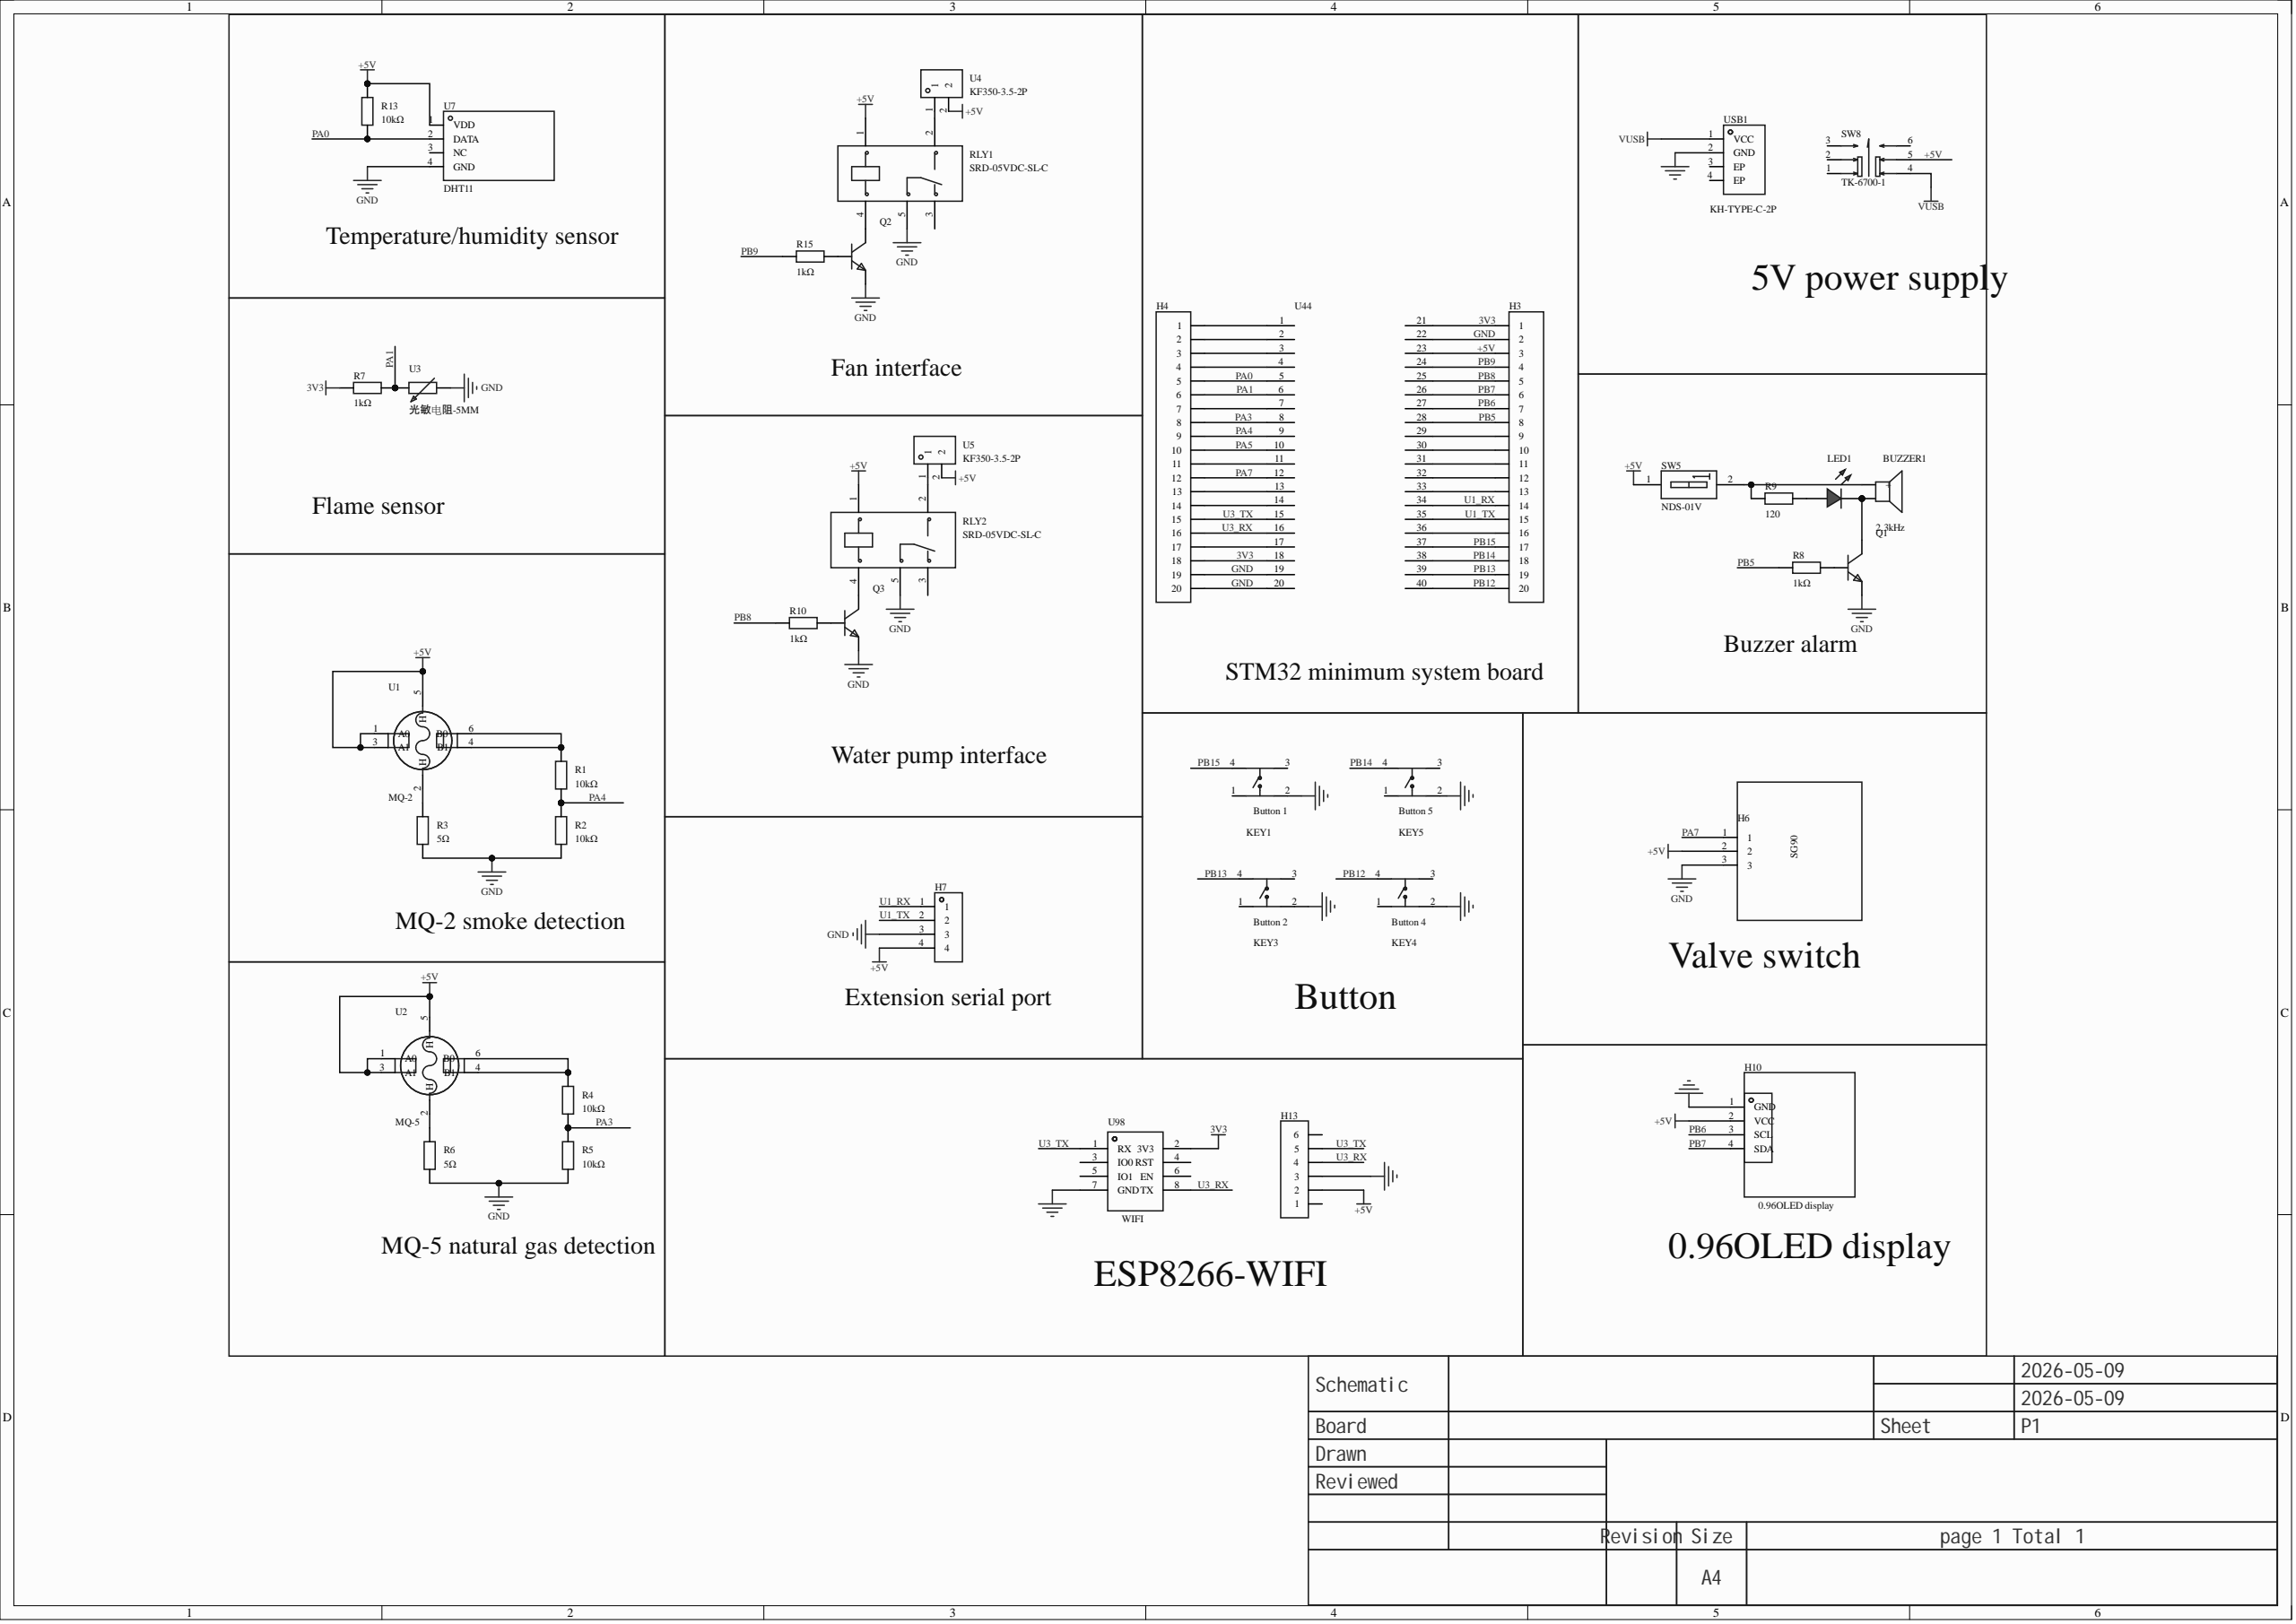Circuit board | Altium Designer | 40 parts | 52 nets
Bill of materials:
Comment,Description,Designator,Footprint,LibRef,Quantity
"2.3kHz","Drive mode: active (built-in driver circuit); construction type: electromagnetic; rated voltage: 5V; frequency: 2.3kHz; sound pressure (SPL): 85dB@5V,10cm;","BUZZER1","BUZ-TH_BD12.0-P7.60-D0.6-FD","TMB12A05_C96093","1"
"","","H3, H4","HDR-TH_20P-P2.54-V-F","HDR-F_2.54_1x20P","2"
"","","H6","HDR-TH_3P-P2.54-V-F","HDR-F_2.54_1x3P","1"
"","","H7","HDR-TH_4P-P2.54-V-F","HDR-F_2.54_1x4P","1"
"2.54-1*4P female","","H10","HDR-TH_4P-P2.54-V-F","0.96OLED屏幕","1"
"","","H13","HDR-TH_6P-P2.54-V-M-1","HDR-M_2.54_1x6P","1"
"Button 1","Circuit structure: SPST; contact rated current: -; button head type: Round Button; button actuation direction: Top Actuated;","KEY1","KEY-TH_4P-L6.0-W6.0-P4.50-LS7.5","按键开关6*6*8","1"
"Button 2","Circuit structure: SPST; contact rated current: -; button head type: Round Button; button actuation direction: Top Actuated;","KEY3","KEY-TH_4P-L6.0-W6.0-P4.50-LS7.5","按键开关6*6*8","1"
"Button 4","Circuit structure: SPST; contact rated current: -; button head type: Round Button; button actuation direction: Top Actuated;","KEY4","KEY-TH_4P-L6.0-W6.0-P4.50-LS7.5","按键开关6*6*8","1"
"Button 5","Circuit structure: SPST; contact rated current: -; button head type: Round Button; button actuation direction: Top Actuated;","KEY5","KEY-TH_4P-L6.0-W6.0-P4.50-LS7.5","按键开关6*6*8","1"
"","","LED1","LED_TH-3mm","LED_TH-R_3mm","1"
"","","Q1, Q2, Q3","S8050_TO_92","S8050_TO_NPN","3"
"10kΩ","","R1, R2, R4, R5, R13","Res_1/4W","Res_AXIAL-1/8W","5"
"5Ω","","R3, R6","Res_1/4W","Res_AXIAL-1/8W","2"
"1kΩ","","R7, R8, R10, R15","Res_1/4W","Res_AXIAL-1/4W, Res_AXIAL-1/8W","4"
"120","","R9","Res_1/4W","Res_AXIAL-1/4W","1"
"SRD-05VDC-SL-C","Coil voltage: 5V; contact form: one changeover: 1C (SPDT); contact rating (resistive load): -; max switching voltage: 250V@AC; max switching current: 15A;","RLY1, RLY2","RELAY-TH_SRD-XXVDC-XL-C","SRD-05VDC-SL-C","2"
"NDS-01V","Forward-throw high lever","SW5","SW-TH_2P-L3.9-W9.9-P2.54-LS7.6","NDS-01V_C501305","1"
"TK-6700-1","","SW8","SW-TH_TK-6700-1","TK-6700-1","1"
"MQ-2","","U1","SENSOR-TH_MQ-2","MQ-2","1"
"MQ-5","","U2","SENSOR-TH_MQ-2","MQ-2","1"
"光敏电阻-5MM","","U3","RES-TH_L4.9-W4.3-P3.4","光敏电阻-5MM","1"
"KF350-3.5-2P","","U4, U5","CONN-TH_P3.50_KF350-3.5-2P","KF350-3.5-2P","2"
"DHT11","","U7","SENSOR-TH_DHT11","DHT11","1"
"","","U44","STM32最小系统板","STM32最小系统板","1"
"","","U98","WiFi封装","WiFi模块","1"
"KH-TYPE-C-2P","Connector type: Type-C; standard: -; male/female: -; number of ports: -; number of contacts: 2P; mounting: -; rated current - power: -; contact material: -; contact plating: -; operating temperature range: -;","USB1","USB-SMD_KH-TYPE-C-2P","KH-TYPE-C-2P","1"
Netlist (Protel format):
[
BUZZER1
BUZ-TH_BD12.0-P7.60-D0.6-FD
2.3kHz



]
[
H3
HDR-TH_20P-P2.54-V-F




]
[
H4
HDR-TH_20P-P2.54-V-F




]
[
H6
HDR-TH_3P-P2.54-V-F




]
[
H7
HDR-TH_4P-P2.54-V-F




]
[
H10
HDR-TH_4P-P2.54-V-F
2.54-1*4P female



]
[
H13
HDR-TH_6P-P2.54-V-M-1




]
[
KEY1
KEY-TH_4P-L6.0-W6.0-P4.50-LS7.5
Button 1



]
[
KEY3
KEY-TH_4P-L6.0-W6.0-P4.50-LS7.5
Button 2



]
[
KEY4
KEY-TH_4P-L6.0-W6.0-P4.50-LS7.5
Button 4



]
[
KEY5
KEY-TH_4P-L6.0-W6.0-P4.50-LS7.5
Button 5



]
[
LED1
LED_TH-3mm




]
[
Q1
S8050_TO_92




]
[
Q2
S8050_TO_92




]
[
Q3
S8050_TO_92




]
[
R1
Res_1/4W
10kΩ



]
[
R2
Res_1/4W
10kΩ



]
[
R3
Res_1/4W
5Ω



]
[
R4
Res_1/4W
10kΩ



]
[
R5
Res_1/4W
10kΩ



]
[
R6
Res_1/4W
5Ω



]
[
R7
Res_1/4W
1kΩ



]
[
R8
Res_1/4W
1kΩ



]
[
R9
Res_1/4W
120



]
[
R10
Res_1/4W
1kΩ



]
[
R13
Res_1/4W
10kΩ



]
[
R15
Res_1/4W
1kΩ



]
[
RLY1
RELAY-TH_SRD-XXVDC-XL-C
SRD-05VDC-SL-C



]
[
RLY2
RELAY-TH_SRD-XXVDC-XL-C
SRD-05VDC-SL-C



]
[
SW5
SW-TH_2P-L3.9-W9.9-P2.54-LS7.6
NDS-01V



]
[
SW8
SW-TH_TK-6700-1
TK-6700-1



]
[
U1
SENSOR-TH_MQ-2
MQ-2



]
[
U2
SENSOR-TH_MQ-2
MQ-5



]
[
U3
RES-TH_L4.9-W4.3-P3.4
光敏电阻-5MM



]
[
U4
CONN-TH_P3.50_KF350-3.5-2P
KF350-3.5-2P



]
[
U5
CONN-TH_P3.50_KF350-3.5-2P
KF350-3.5-2P



]
[
U7
SENSOR-TH_DHT11
DHT11



]
[
U44
STM32最小系统板




]
[
U98
WiFi封装




]
[
USB1
USB-SMD_KH-TYPE-C-2P
KH-TYPE-C-2P



]
(
VUSB
SW8-4
USB1-1
)
(
U3_TX
H4-15
H13-5
U44-15
U98-1
)
(
U3_RX
H4-16
H13-4
U44-16
U98-8
)
(
U1_TX
H3-15
H7-2
U44-35
)
(
U1_RX
H3-14
H7-1
U44-34
)
(
PB15
H3-17
KEY1-4
U44-37
)
(
PB14
H3-18
KEY5-4
U44-38
)
(
PB13
H3-19
KEY3-4
U44-39
)
(
PB12
H3-20
KEY4-4
U44-40
)
(
PB9
H3-4
R15-1
U44-24
)
(
PB8
H3-5
R10-1
U44-25
)
(
PB7
H3-6
H10-4
U44-26
)
(
PB6
H3-7
H10-3
U44-27
)
(
PB5
H3-8
R8-1
U44-28
)
(
PA7
H4-12
H6-1
U44-12
)
(
PA5
H4-10
U44-10
)
(
PA4
H4-9
R1-1
R2-2
U44-9
)
(
PA3
H4-8
R4-1
R5-2
U44-8
)
(
PA1
H4-6
R7-2
U3-2
U44-6
)
(
PA0
H4-5
R13-1
U7-2
U44-5
)
(
NetRLY2_2
RLY2-2
U5-1
)
(
NetRLY1_2
RLY1-2
U4-1
)
(
NetR6_2
R6-2
U2-2
)
(
NetR4_2
R4-2
U2-4
U2-6
)
(
NetR3_2
R3-2
U1-2
)
(
NetR1_2
R1-2
U1-4
U1-6
)
(
NetQ3_3
Q3-3
RLY2-4
)
(
NetQ3_2
Q3-2
R10-2
)
(
NetQ2_3
Q2-3
RLY1-4
)
(
NetQ2_2
Q2-2
R15-2
)
(
NetQ1_2
Q1-2
R8-2
)
(
NetLED1_1
LED1-1
R9-2
)
(
NetH4_17
H4-17
U44-17
)
(
NetH4_14
H4-14
U44-14
)
(
NetH4_13
H4-13
U44-13
)
(
NetH4_11
H4-11
U44-11
)
(
NetH4_7
H4-7
U44-7
)
(
NetH4_4
H4-4
U44-4
)
(
NetH4_3
H4-3
U44-3
)
(
NetH4_2
H4-2
U44-2
)
(
NetH4_1
H4-1
U44-1
)
(
NetH3_16
H3-16
U44-36
)
(
NetH3_13
H3-13
U44-33
)
(
NetH3_12
H3-12
U44-32
)
(
NetH3_11
H3-11
U44-31
)
(
NetH3_10
H3-10
U44-30
)
(
NetH3_9
H3-9
U44-29
)
(
NetBUZZER1_2
BUZZER1-2
LED1-2
Q1-3
)
(
NetBUZZER1_1
BUZZER1-1
R9-1
SW5-2
)
(
GND
H3-2
H4-19
H4-20
H6-3
H7-3
H10-1
H13-3
KEY1-2
KEY3-2
KEY4-2
KEY5-2
Q1-1
Q2-1
Q3-1
R2-1
R3-1
R5-1
R6-1
RLY1-5
RLY2-5
U3-1
U7-4
U44-19
U44-20
U44-22
U98-7
USB1-2
)
(
+5V
H3-3
H6-2
H7-4
H10-2
H13-2
R13-2
RLY1-1
RLY2-1
SW5-1
SW8-5
U1-1
U1-3
U1-5
U2-1
U2-3
U2-5
U4-2
U5-2
U7-1
U44-23
)
(
3V3
H3-1
H4-18
R7-1
U44-18
U44-21
U98-2
)